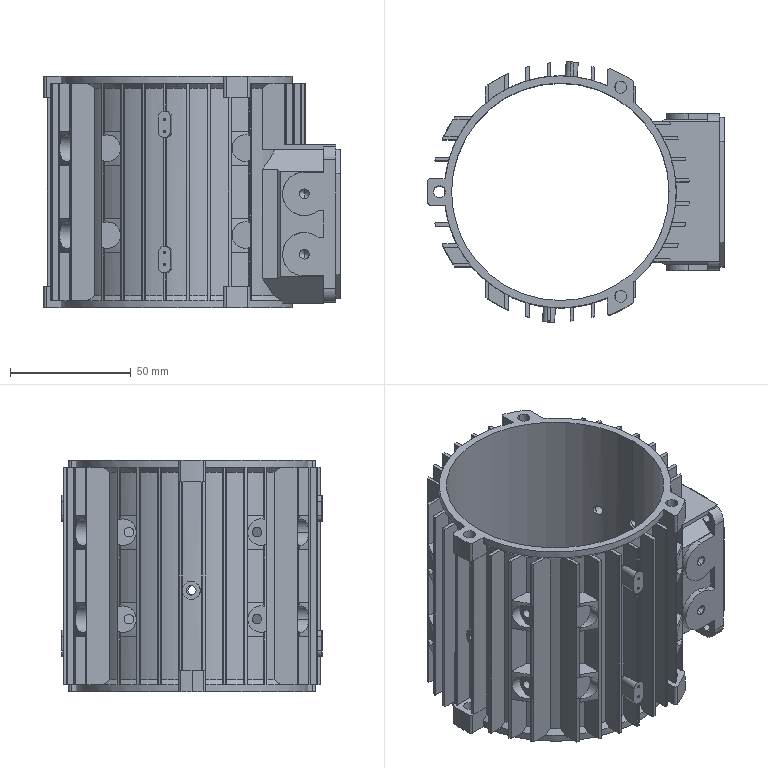Part | SolidWorks | features BaseBody 5 | 5 solids | 761 faces | box 123 x 107.955 x 96 mm | volume 90735 mm3 | cylinder 347 | plane 324 | cone 90 | commonest cylinder face diameters 0.4 x88 107 x60 4 x52 92 x46 5 x20 11 x18